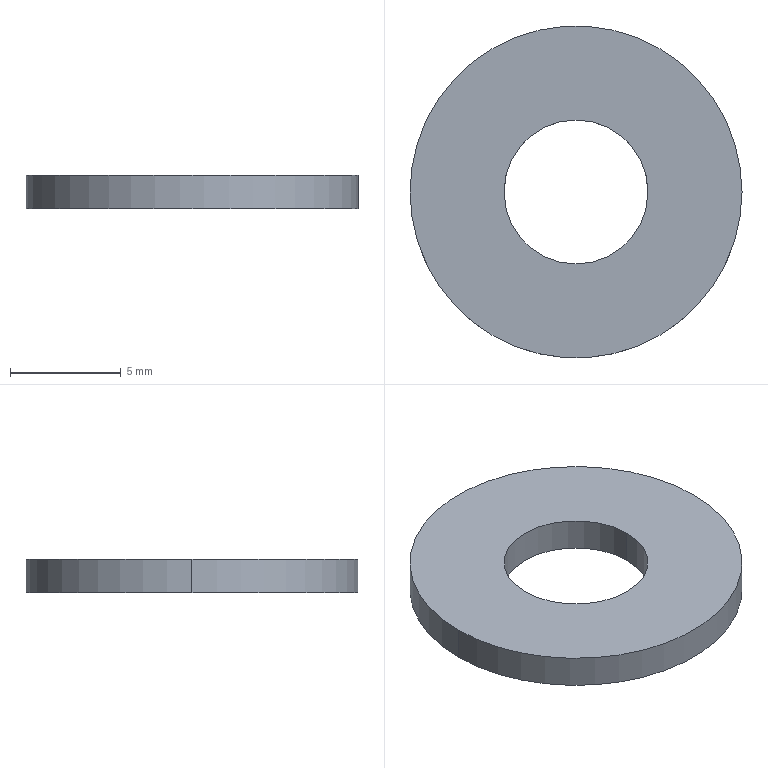Part | STEP file | Washer | 1 solid | 6 faces | box 15 x 15 x 1.5 mm | volume 215.297 mm3 | cylinder 4 | plane 2 | commonest cylinder face diameters 6.5 x2 15 x2
STEP:
#1=CARTESIAN_POINT('',(0.,0.,0.));
#2=DIRECTION('',(0.,0.,1.));
#3=DIRECTION('',(1.,0.,0.));
#4=AXIS2_PLACEMENT_3D('',#1,#2,#3);
#5=CARTESIAN_POINT('',(-3.25,0.,1.5));
#6=VERTEX_POINT('',#5);
#7=CARTESIAN_POINT('',(-3.25,0.,0.));
#8=VERTEX_POINT('',#7);
#9=CARTESIAN_POINT('',(-3.25,0.,1.5));
#10=DIRECTION('',(0.,0.,-1.));
#11=VECTOR('',#10,1.);
#12=LINE('',#9,#11);
#13=CARTESIAN_POINT('',(0.,0.,1.5));
#14=DIRECTION('',(0.,0.,-1.));
#15=DIRECTION('',(-1.,0.,0.));
#16=AXIS2_PLACEMENT_3D('',#13,#14,#15);
#17=CYLINDRICAL_SURFACE('',#16,3.25);
#18=CARTESIAN_POINT('',(6.283,0.));
#19=DIRECTION('',(0.,1.));
#20=VECTOR('',#19,1.);
#21=LINE('',#18,#20);
#22=(GEOMETRIC_REPRESENTATION_CONTEXT(2)PARAMETRIC_REPRESENTATION_CONTEXT()REPRESENTATION_CONTEXT('',''));
#23=DEFINITIONAL_REPRESENTATION('',(#21),#22);
#24=PCURVE('',#17,#23);
#25=CARTESIAN_POINT('',(0.,0.,1.5));
#26=DIRECTION('',(0.,0.,-1.));
#27=DIRECTION('',(-1.,0.,0.));
#28=AXIS2_PLACEMENT_3D('',#25,#26,#27);
#29=CYLINDRICAL_SURFACE('',#28,3.25);
#30=CARTESIAN_POINT('',(0.,0.));
#31=DIRECTION('',(0.,1.));
#32=VECTOR('',#31,1.);
#33=LINE('',#30,#32);
#34=(GEOMETRIC_REPRESENTATION_CONTEXT(2)PARAMETRIC_REPRESENTATION_CONTEXT()REPRESENTATION_CONTEXT('',''));
#35=DEFINITIONAL_REPRESENTATION('',(#33),#34);
#36=PCURVE('',#29,#35);
#37=SURFACE_CURVE('',#12,(#24,#36),.PCURVE_S1.);
#38=EDGE_CURVE('',#6,#8,#37,.T.);
#39=ORIENTED_EDGE('',*,*,#38,.T.);
#40=CARTESIAN_POINT('',(3.25,0.,0.));
#41=VERTEX_POINT('',#40);
#42=CARTESIAN_POINT('',(0.,0.,0.));
#43=DIRECTION('',(0.,0.,1.));
#44=DIRECTION('',(1.,0.,0.));
#45=AXIS2_PLACEMENT_3D('',#42,#43,#44);
#46=CIRCLE('',#45,3.25);
#47=CARTESIAN_POINT('',(9.425,1.5));
#48=DIRECTION('',(-1.,0.));
#49=VECTOR('',#48,1.);
#50=LINE('',#47,#49);
#51=(GEOMETRIC_REPRESENTATION_CONTEXT(2)PARAMETRIC_REPRESENTATION_CONTEXT()REPRESENTATION_CONTEXT('',''));
#52=DEFINITIONAL_REPRESENTATION('',(#50),#51);
#53=PCURVE('',#17,#52);
#54=CARTESIAN_POINT('',(0.,0.,0.));
#55=DIRECTION('',(0.,0.,1.));
#56=DIRECTION('',(1.,0.,0.));
#57=AXIS2_PLACEMENT_3D('',#54,#55,#56);
#58=PLANE('',#57);
#59=CARTESIAN_POINT('',(0.,0.));
#60=DIRECTION('',(1.,0.));
#61=AXIS2_PLACEMENT_2D('',#59,#60);
#62=CIRCLE('',#61,3.25);
#63=(GEOMETRIC_REPRESENTATION_CONTEXT(2)PARAMETRIC_REPRESENTATION_CONTEXT()REPRESENTATION_CONTEXT('',''));
#64=DEFINITIONAL_REPRESENTATION('',(#62),#63);
#65=PCURVE('',#58,#64);
#66=SURFACE_CURVE('',#46,(#53,#65),.PCURVE_S1.);
#67=EDGE_CURVE('',#8,#41,#66,.T.);
#68=ORIENTED_EDGE('',*,*,#67,.T.);
#69=CARTESIAN_POINT('',(3.25,0.,1.5));
#70=VERTEX_POINT('',#69);
#71=CARTESIAN_POINT('',(3.25,0.,1.5));
#72=DIRECTION('',(0.,0.,-1.));
#73=VECTOR('',#72,1.);
#74=LINE('',#71,#73);
#75=CARTESIAN_POINT('',(3.142,0.));
#76=DIRECTION('',(0.,1.));
#77=VECTOR('',#76,1.);
#78=LINE('',#75,#77);
#79=(GEOMETRIC_REPRESENTATION_CONTEXT(2)PARAMETRIC_REPRESENTATION_CONTEXT()REPRESENTATION_CONTEXT('',''));
#80=DEFINITIONAL_REPRESENTATION('',(#78),#79);
#81=PCURVE('',#17,#80);
#82=CARTESIAN_POINT('',(3.142,0.));
#83=DIRECTION('',(0.,1.));
#84=VECTOR('',#83,1.);
#85=LINE('',#82,#84);
#86=(GEOMETRIC_REPRESENTATION_CONTEXT(2)PARAMETRIC_REPRESENTATION_CONTEXT()REPRESENTATION_CONTEXT('',''));
#87=DEFINITIONAL_REPRESENTATION('',(#85),#86);
#88=PCURVE('',#29,#87);
#89=SURFACE_CURVE('',#74,(#81,#88),.PCURVE_S1.);
#90=EDGE_CURVE('',#70,#41,#89,.T.);
#91=ORIENTED_EDGE('',*,*,#90,.F.);
#92=CARTESIAN_POINT('',(0.,0.,1.5));
#93=DIRECTION('',(0.,0.,1.));
#94=DIRECTION('',(1.,0.,0.));
#95=AXIS2_PLACEMENT_3D('',#92,#93,#94);
#96=CIRCLE('',#95,3.25);
#97=CARTESIAN_POINT('',(9.425,0.));
#98=DIRECTION('',(-1.,0.));
#99=VECTOR('',#98,1.);
#100=LINE('',#97,#99);
#101=(GEOMETRIC_REPRESENTATION_CONTEXT(2)PARAMETRIC_REPRESENTATION_CONTEXT()REPRESENTATION_CONTEXT('',''));
#102=DEFINITIONAL_REPRESENTATION('',(#100),#101);
#103=PCURVE('',#17,#102);
#104=CARTESIAN_POINT('',(0.,0.,1.5));
#105=DIRECTION('',(0.,0.,1.));
#106=DIRECTION('',(1.,0.,0.));
#107=AXIS2_PLACEMENT_3D('',#104,#105,#106);
#108=PLANE('',#107);
#109=CARTESIAN_POINT('',(0.,0.));
#110=DIRECTION('',(1.,0.));
#111=AXIS2_PLACEMENT_2D('',#109,#110);
#112=CIRCLE('',#111,3.25);
#113=(GEOMETRIC_REPRESENTATION_CONTEXT(2)PARAMETRIC_REPRESENTATION_CONTEXT()REPRESENTATION_CONTEXT('',''));
#114=DEFINITIONAL_REPRESENTATION('',(#112),#113);
#115=PCURVE('',#108,#114);
#116=SURFACE_CURVE('',#96,(#103,#115),.PCURVE_S1.);
#117=EDGE_CURVE('',#6,#70,#116,.T.);
#118=ORIENTED_EDGE('',*,*,#117,.F.);
#119=EDGE_LOOP('',(#39,#68,#91,#118));
#120=FACE_BOUND('',#119,.F.);
#121=ADVANCED_FACE('',(#120),#17,.F.);
#122=CARTESIAN_POINT('',(7.5,0.,1.5));
#123=VERTEX_POINT('',#122);
#124=CARTESIAN_POINT('',(-7.5,0.,1.5));
#125=VERTEX_POINT('',#124);
#126=CARTESIAN_POINT('',(0.,0.,1.5));
#127=DIRECTION('',(0.,0.,1.));
#128=DIRECTION('',(1.,0.,0.));
#129=AXIS2_PLACEMENT_3D('',#126,#127,#128);
#130=CIRCLE('',#129,7.5);
#131=CARTESIAN_POINT('',(0.,0.,1.5));
#132=DIRECTION('',(0.,0.,-1.));
#133=DIRECTION('',(-1.,0.,0.));
#134=AXIS2_PLACEMENT_3D('',#131,#132,#133);
#135=CYLINDRICAL_SURFACE('',#134,7.5);
#136=CARTESIAN_POINT('',(3.142,0.));
#137=DIRECTION('',(-1.,0.));
#138=VECTOR('',#137,1.);
#139=LINE('',#136,#138);
#140=(GEOMETRIC_REPRESENTATION_CONTEXT(2)PARAMETRIC_REPRESENTATION_CONTEXT()REPRESENTATION_CONTEXT('',''));
#141=DEFINITIONAL_REPRESENTATION('',(#139),#140);
#142=PCURVE('',#135,#141);
#143=CARTESIAN_POINT('',(0.,0.));
#144=DIRECTION('',(1.,0.));
#145=AXIS2_PLACEMENT_2D('',#143,#144);
#146=CIRCLE('',#145,7.5);
#147=(GEOMETRIC_REPRESENTATION_CONTEXT(2)PARAMETRIC_REPRESENTATION_CONTEXT()REPRESENTATION_CONTEXT('',''));
#148=DEFINITIONAL_REPRESENTATION('',(#146),#147);
#149=PCURVE('',#108,#148);
#150=SURFACE_CURVE('',#130,(#142,#149),.PCURVE_S1.);
#151=EDGE_CURVE('',#123,#125,#150,.T.);
#152=ORIENTED_EDGE('',*,*,#151,.F.);
#153=CARTESIAN_POINT('',(7.5,0.,0.));
#154=VERTEX_POINT('',#153);
#155=CARTESIAN_POINT('',(7.5,0.,1.5));
#156=DIRECTION('',(0.,0.,-1.));
#157=VECTOR('',#156,1.);
#158=LINE('',#155,#157);
#159=CARTESIAN_POINT('',(3.142,0.));
#160=DIRECTION('',(0.,1.));
#161=VECTOR('',#160,1.);
#162=LINE('',#159,#161);
#163=(GEOMETRIC_REPRESENTATION_CONTEXT(2)PARAMETRIC_REPRESENTATION_CONTEXT()REPRESENTATION_CONTEXT('',''));
#164=DEFINITIONAL_REPRESENTATION('',(#162),#163);
#165=PCURVE('',#135,#164);
#166=CARTESIAN_POINT('',(0.,0.,1.5));
#167=DIRECTION('',(0.,0.,-1.));
#168=DIRECTION('',(-1.,0.,0.));
#169=AXIS2_PLACEMENT_3D('',#166,#167,#168);
#170=CYLINDRICAL_SURFACE('',#169,7.5);
#171=CARTESIAN_POINT('',(3.142,0.));
#172=DIRECTION('',(0.,1.));
#173=VECTOR('',#172,1.);
#174=LINE('',#171,#173);
#175=(GEOMETRIC_REPRESENTATION_CONTEXT(2)PARAMETRIC_REPRESENTATION_CONTEXT()REPRESENTATION_CONTEXT('',''));
#176=DEFINITIONAL_REPRESENTATION('',(#174),#175);
#177=PCURVE('',#170,#176);
#178=SURFACE_CURVE('',#158,(#165,#177),.PCURVE_S1.);
#179=EDGE_CURVE('',#123,#154,#178,.T.);
#180=ORIENTED_EDGE('',*,*,#179,.T.);
#181=CARTESIAN_POINT('',(-7.5,0.,0.));
#182=VERTEX_POINT('',#181);
#183=CARTESIAN_POINT('',(0.,0.,0.));
#184=DIRECTION('',(0.,0.,1.));
#185=DIRECTION('',(1.,0.,0.));
#186=AXIS2_PLACEMENT_3D('',#183,#184,#185);
#187=CIRCLE('',#186,7.5);
#188=CARTESIAN_POINT('',(3.142,1.5));
#189=DIRECTION('',(-1.,0.));
#190=VECTOR('',#189,1.);
#191=LINE('',#188,#190);
#192=(GEOMETRIC_REPRESENTATION_CONTEXT(2)PARAMETRIC_REPRESENTATION_CONTEXT()REPRESENTATION_CONTEXT('',''));
#193=DEFINITIONAL_REPRESENTATION('',(#191),#192);
#194=PCURVE('',#135,#193);
#195=CARTESIAN_POINT('',(0.,0.));
#196=DIRECTION('',(1.,0.));
#197=AXIS2_PLACEMENT_2D('',#195,#196);
#198=CIRCLE('',#197,7.5);
#199=(GEOMETRIC_REPRESENTATION_CONTEXT(2)PARAMETRIC_REPRESENTATION_CONTEXT()REPRESENTATION_CONTEXT('',''));
#200=DEFINITIONAL_REPRESENTATION('',(#198),#199);
#201=PCURVE('',#58,#200);
#202=SURFACE_CURVE('',#187,(#194,#201),.PCURVE_S1.);
#203=EDGE_CURVE('',#154,#182,#202,.T.);
#204=ORIENTED_EDGE('',*,*,#203,.T.);
#205=CARTESIAN_POINT('',(-7.5,0.,1.5));
#206=DIRECTION('',(0.,0.,-1.));
#207=VECTOR('',#206,1.);
#208=LINE('',#205,#207);
#209=CARTESIAN_POINT('',(0.,0.));
#210=DIRECTION('',(0.,1.));
#211=VECTOR('',#210,1.);
#212=LINE('',#209,#211);
#213=(GEOMETRIC_REPRESENTATION_CONTEXT(2)PARAMETRIC_REPRESENTATION_CONTEXT()REPRESENTATION_CONTEXT('',''));
#214=DEFINITIONAL_REPRESENTATION('',(#212),#213);
#215=PCURVE('',#135,#214);
#216=CARTESIAN_POINT('',(6.283,0.));
#217=DIRECTION('',(0.,1.));
#218=VECTOR('',#217,1.);
#219=LINE('',#216,#218);
#220=(GEOMETRIC_REPRESENTATION_CONTEXT(2)PARAMETRIC_REPRESENTATION_CONTEXT()REPRESENTATION_CONTEXT('',''));
#221=DEFINITIONAL_REPRESENTATION('',(#219),#220);
#222=PCURVE('',#170,#221);
#223=SURFACE_CURVE('',#208,(#215,#222),.PCURVE_S1.);
#224=EDGE_CURVE('',#125,#182,#223,.T.);
#225=ORIENTED_EDGE('',*,*,#224,.F.);
#226=EDGE_LOOP('',(#152,#180,#204,#225));
#227=FACE_BOUND('',#226,.T.);
#228=ADVANCED_FACE('',(#227),#135,.T.);
#229=CARTESIAN_POINT('',(0.,0.,1.5));
#230=DIRECTION('',(0.,0.,1.));
#231=DIRECTION('',(1.,0.,0.));
#232=AXIS2_PLACEMENT_3D('',#229,#230,#231);
#233=CIRCLE('',#232,7.5);
#234=CARTESIAN_POINT('',(0.,0.));
#235=DIRECTION('',(1.,0.));
#236=AXIS2_PLACEMENT_2D('',#234,#235);
#237=CIRCLE('',#236,7.5);
#238=(GEOMETRIC_REPRESENTATION_CONTEXT(2)PARAMETRIC_REPRESENTATION_CONTEXT()REPRESENTATION_CONTEXT('',''));
#239=DEFINITIONAL_REPRESENTATION('',(#237),#238);
#240=PCURVE('',#108,#239);
#241=CARTESIAN_POINT('',(9.425,0.));
#242=DIRECTION('',(-1.,0.));
#243=VECTOR('',#242,1.);
#244=LINE('',#241,#243);
#245=(GEOMETRIC_REPRESENTATION_CONTEXT(2)PARAMETRIC_REPRESENTATION_CONTEXT()REPRESENTATION_CONTEXT('',''));
#246=DEFINITIONAL_REPRESENTATION('',(#244),#245);
#247=PCURVE('',#170,#246);
#248=SURFACE_CURVE('',#233,(#240,#247),.PCURVE_S1.);
#249=EDGE_CURVE('',#125,#123,#248,.T.);
#250=ORIENTED_EDGE('',*,*,#249,.T.);
#251=ORIENTED_EDGE('',*,*,#151,.T.);
#252=EDGE_LOOP('',(#250,#251));
#253=FACE_BOUND('',#252,.T.);
#254=ORIENTED_EDGE('',*,*,#117,.F.);
#255=CARTESIAN_POINT('',(0.,0.,1.5));
#256=DIRECTION('',(0.,0.,1.));
#257=DIRECTION('',(1.,0.,0.));
#258=AXIS2_PLACEMENT_3D('',#255,#256,#257);
#259=CIRCLE('',#258,3.25);
#260=CARTESIAN_POINT('',(0.,0.));
#261=DIRECTION('',(1.,0.));
#262=AXIS2_PLACEMENT_2D('',#260,#261);
#263=CIRCLE('',#262,3.25);
#264=(GEOMETRIC_REPRESENTATION_CONTEXT(2)PARAMETRIC_REPRESENTATION_CONTEXT()REPRESENTATION_CONTEXT('',''));
#265=DEFINITIONAL_REPRESENTATION('',(#263),#264);
#266=PCURVE('',#108,#265);
#267=CARTESIAN_POINT('',(3.142,0.));
#268=DIRECTION('',(-1.,0.));
#269=VECTOR('',#268,1.);
#270=LINE('',#267,#269);
#271=(GEOMETRIC_REPRESENTATION_CONTEXT(2)PARAMETRIC_REPRESENTATION_CONTEXT()REPRESENTATION_CONTEXT('',''));
#272=DEFINITIONAL_REPRESENTATION('',(#270),#271);
#273=PCURVE('',#29,#272);
#274=SURFACE_CURVE('',#259,(#266,#273),.PCURVE_S1.);
#275=EDGE_CURVE('',#70,#6,#274,.T.);
#276=ORIENTED_EDGE('',*,*,#275,.F.);
#277=EDGE_LOOP('',(#254,#276));
#278=FACE_BOUND('',#277,.T.);
#279=ADVANCED_FACE('',(#253,#278),#108,.T.);
#280=CARTESIAN_POINT('',(0.,0.,0.));
#281=DIRECTION('',(0.,0.,1.));
#282=DIRECTION('',(1.,0.,0.));
#283=AXIS2_PLACEMENT_3D('',#280,#281,#282);
#284=CIRCLE('',#283,7.5);
#285=CARTESIAN_POINT('',(0.,0.));
#286=DIRECTION('',(1.,0.));
#287=AXIS2_PLACEMENT_2D('',#285,#286);
#288=CIRCLE('',#287,7.5);
#289=(GEOMETRIC_REPRESENTATION_CONTEXT(2)PARAMETRIC_REPRESENTATION_CONTEXT()REPRESENTATION_CONTEXT('',''));
#290=DEFINITIONAL_REPRESENTATION('',(#288),#289);
#291=PCURVE('',#58,#290);
#292=CARTESIAN_POINT('',(9.425,1.5));
#293=DIRECTION('',(-1.,0.));
#294=VECTOR('',#293,1.);
#295=LINE('',#292,#294);
#296=(GEOMETRIC_REPRESENTATION_CONTEXT(2)PARAMETRIC_REPRESENTATION_CONTEXT()REPRESENTATION_CONTEXT('',''));
#297=DEFINITIONAL_REPRESENTATION('',(#295),#296);
#298=PCURVE('',#170,#297);
#299=SURFACE_CURVE('',#284,(#291,#298),.PCURVE_S1.);
#300=EDGE_CURVE('',#182,#154,#299,.T.);
#301=ORIENTED_EDGE('',*,*,#300,.F.);
#302=ORIENTED_EDGE('',*,*,#203,.F.);
#303=EDGE_LOOP('',(#301,#302));
#304=FACE_BOUND('',#303,.T.);
#305=ORIENTED_EDGE('',*,*,#67,.T.);
#306=CARTESIAN_POINT('',(0.,0.,0.));
#307=DIRECTION('',(0.,0.,1.));
#308=DIRECTION('',(1.,0.,0.));
#309=AXIS2_PLACEMENT_3D('',#306,#307,#308);
#310=CIRCLE('',#309,3.25);
#311=CARTESIAN_POINT('',(0.,0.));
#312=DIRECTION('',(1.,0.));
#313=AXIS2_PLACEMENT_2D('',#311,#312);
#314=CIRCLE('',#313,3.25);
#315=(GEOMETRIC_REPRESENTATION_CONTEXT(2)PARAMETRIC_REPRESENTATION_CONTEXT()REPRESENTATION_CONTEXT('',''));
#316=DEFINITIONAL_REPRESENTATION('',(#314),#315);
#317=PCURVE('',#58,#316);
#318=CARTESIAN_POINT('',(3.142,1.5));
#319=DIRECTION('',(-1.,0.));
#320=VECTOR('',#319,1.);
#321=LINE('',#318,#320);
#322=(GEOMETRIC_REPRESENTATION_CONTEXT(2)PARAMETRIC_REPRESENTATION_CONTEXT()REPRESENTATION_CONTEXT('',''));
#323=DEFINITIONAL_REPRESENTATION('',(#321),#322);
#324=PCURVE('',#29,#323);
#325=SURFACE_CURVE('',#310,(#317,#324),.PCURVE_S1.);
#326=EDGE_CURVE('',#41,#8,#325,.T.);
#327=ORIENTED_EDGE('',*,*,#326,.T.);
#328=EDGE_LOOP('',(#305,#327));
#329=FACE_BOUND('',#328,.T.);
#330=ADVANCED_FACE('',(#304,#329),#58,.F.);
#331=ORIENTED_EDGE('',*,*,#179,.F.);
#332=ORIENTED_EDGE('',*,*,#249,.F.);
#333=ORIENTED_EDGE('',*,*,#224,.T.);
#334=ORIENTED_EDGE('',*,*,#300,.T.);
#335=EDGE_LOOP('',(#331,#332,#333,#334));
#336=FACE_BOUND('',#335,.T.);
#337=ADVANCED_FACE('',(#336),#170,.T.);
#338=ORIENTED_EDGE('',*,*,#326,.T.);
#339=ORIENTED_EDGE('',*,*,#38,.F.);
#340=ORIENTED_EDGE('',*,*,#275,.F.);
#341=ORIENTED_EDGE('',*,*,#90,.T.);
#342=EDGE_LOOP('',(#338,#339,#340,#341));
#343=FACE_BOUND('',#342,.F.);
#344=ADVANCED_FACE('',(#343),#29,.F.);
#345=CLOSED_SHELL('',(#121,#228,#279,#330,#337,#344));
#346=MANIFOLD_SOLID_BREP('',#345);
#347=(LENGTH_UNIT()NAMED_UNIT(*)SI_UNIT(.MILLI.,.METRE.));
#348=UNCERTAINTY_MEASURE_WITH_UNIT(LENGTH_MEASURE(0.0000001),#347,'','');
#349=(NAMED_UNIT(*)PLANE_ANGLE_UNIT()SI_UNIT($,.RADIAN.));
#350=(NAMED_UNIT(*)SI_UNIT($,.STERADIAN.)SOLID_ANGLE_UNIT());
#351=(GEOMETRIC_REPRESENTATION_CONTEXT(3)GLOBAL_UNCERTAINTY_ASSIGNED_CONTEXT((#348))GLOBAL_UNIT_ASSIGNED_CONTEXT((#347,#349,#350))REPRESENTATION_CONTEXT('',''));
#352=ADVANCED_BREP_SHAPE_REPRESENTATION('',(#4,#346),#351);